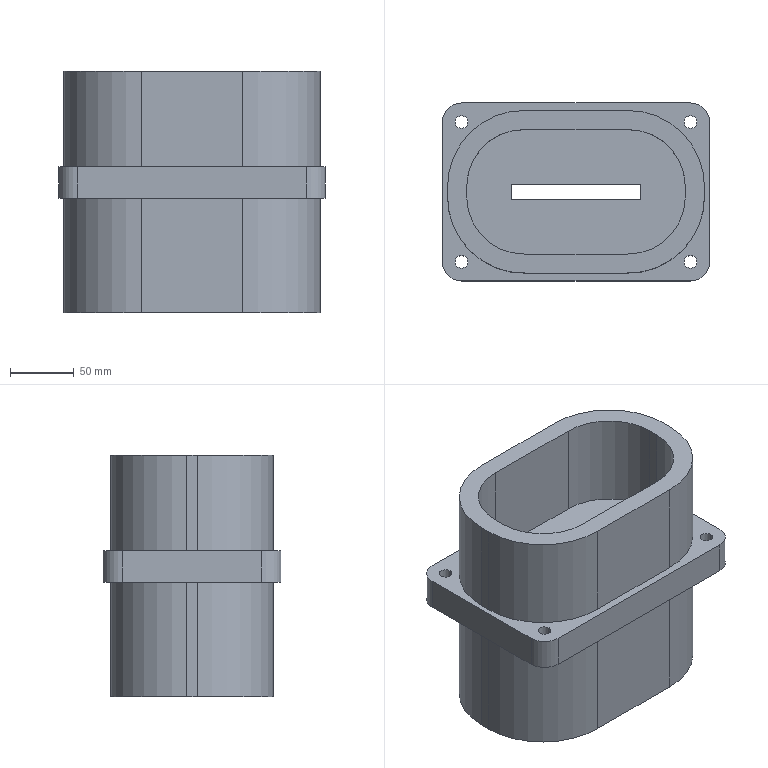Part | STEP file | Bushing 110 x 180 | 1 solid | 58 faces | box 210 x 140 x 190 mm | volume 1953392 mm3 | plane 30 | cylinder 28 | commonest cylinder face diameters 10 x8 30 x4 89.902 x4 90 x4 119.902 x4 120 x4